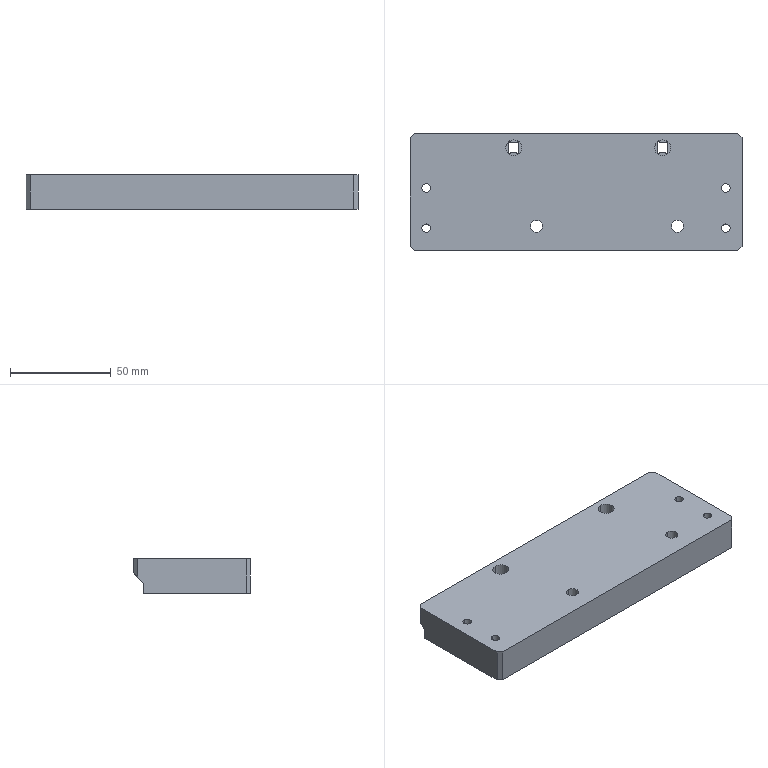Part | 1 solid | 78 faces | box 165 x 58 x 17 mm | volume 150320 mm3 | cylinder 42 | plane 36 | commonest cylinder face diameters 1 x12 2 x8 4.2 x8 14.5 x6 6 x4 8 x4